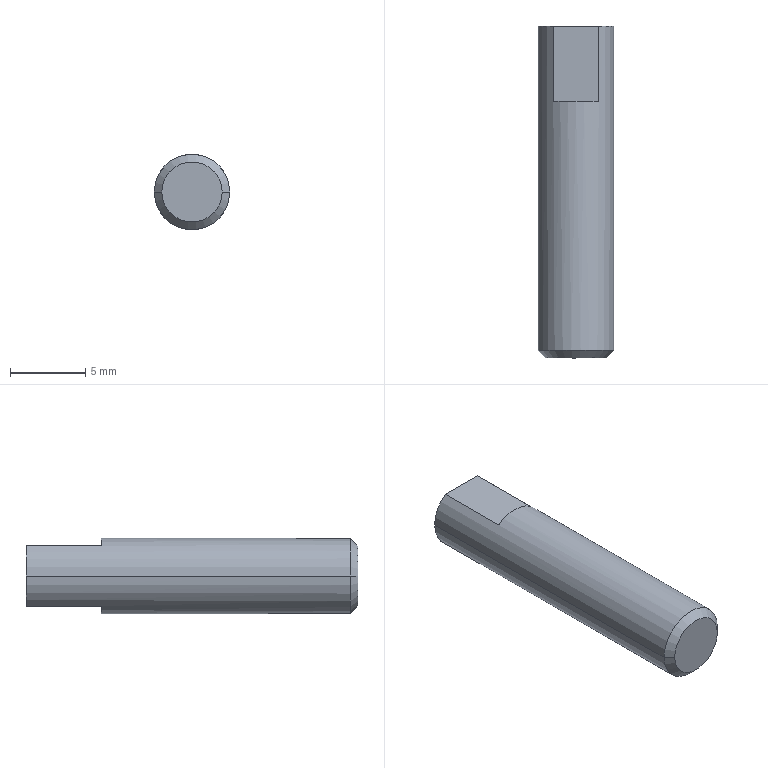Part | STEP file | BU-C08b-1 | 1 solid | 10 faces | box 5 x 22 x 5 mm | volume 419.918 mm3 | plane 6 | cone 2 | cylinder 2 | commonest cylinder face diameters 5 x2
STEP:
#1=CARTESIAN_POINT('',(0.,0.,0.));
#2=DIRECTION('',(0.,0.,1.));
#3=DIRECTION('',(1.,0.,0.));
#4=AXIS2_PLACEMENT_3D('',#1,#2,#3);
#5=CARTESIAN_POINT('',(2.,0.,0.));
#6=VERTEX_POINT('',#5);
#7=CARTESIAN_POINT('',(-2.,0.,0.));
#8=VERTEX_POINT('',#7);
#9=CARTESIAN_POINT('',(0.,0.,0.));
#10=DIRECTION('',(0.,-1.,0.));
#11=DIRECTION('',(1.,0.,0.));
#12=AXIS2_PLACEMENT_3D('',#9,#10,#11);
#13=CIRCLE('',#12,2.);
#14=CARTESIAN_POINT('',(0.,0.,0.));
#15=DIRECTION('',(0.,1.,0.));
#16=DIRECTION('',(-1.,0.,0.));
#17=AXIS2_PLACEMENT_3D('',#14,#15,#16);
#18=CONICAL_SURFACE('',#17,2.,0.7854);
#19=CARTESIAN_POINT('',(3.142,0.));
#20=DIRECTION('',(-1.,0.));
#21=VECTOR('',#20,1.);
#22=LINE('',#19,#21);
#23=(GEOMETRIC_REPRESENTATION_CONTEXT(2)PARAMETRIC_REPRESENTATION_CONTEXT()REPRESENTATION_CONTEXT('',''));
#24=DEFINITIONAL_REPRESENTATION('',(#22),#23);
#25=PCURVE('',#18,#24);
#26=CARTESIAN_POINT('',(0.,0.,0.));
#27=DIRECTION('',(0.,-1.,0.));
#28=DIRECTION('',(1.,0.,0.));
#29=AXIS2_PLACEMENT_3D('',#26,#27,#28);
#30=PLANE('',#29);
#31=CARTESIAN_POINT('',(0.,0.));
#32=DIRECTION('',(1.,0.));
#33=AXIS2_PLACEMENT_2D('',#31,#32);
#34=CIRCLE('',#33,2.);
#35=(GEOMETRIC_REPRESENTATION_CONTEXT(2)PARAMETRIC_REPRESENTATION_CONTEXT()REPRESENTATION_CONTEXT('',''));
#36=DEFINITIONAL_REPRESENTATION('',(#34),#35);
#37=PCURVE('',#30,#36);
#38=SURFACE_CURVE('',#13,(#25,#37),.PCURVE_S1.);
#39=EDGE_CURVE('',#6,#8,#38,.T.);
#40=ORIENTED_EDGE('',*,*,#39,.F.);
#41=CARTESIAN_POINT('',(2.5,0.5,0.));
#42=VERTEX_POINT('',#41);
#43=CARTESIAN_POINT('',(2.,0.,0.));
#44=DIRECTION('',(0.7071,0.7071,0.));
#45=VECTOR('',#44,1.);
#46=LINE('',#43,#45);
#47=CARTESIAN_POINT('',(3.142,0.));
#48=DIRECTION('',(0.,1.));
#49=VECTOR('',#48,1.);
#50=LINE('',#47,#49);
#51=(GEOMETRIC_REPRESENTATION_CONTEXT(2)PARAMETRIC_REPRESENTATION_CONTEXT()REPRESENTATION_CONTEXT('',''));
#52=DEFINITIONAL_REPRESENTATION('',(#50),#51);
#53=PCURVE('',#18,#52);
#54=CARTESIAN_POINT('',(0.,0.,0.));
#55=DIRECTION('',(0.,1.,0.));
#56=DIRECTION('',(-1.,0.,0.));
#57=AXIS2_PLACEMENT_3D('',#54,#55,#56);
#58=CONICAL_SURFACE('',#57,2.,0.7854);
#59=CARTESIAN_POINT('',(3.142,0.));
#60=DIRECTION('',(0.,1.));
#61=VECTOR('',#60,1.);
#62=LINE('',#59,#61);
#63=(GEOMETRIC_REPRESENTATION_CONTEXT(2)PARAMETRIC_REPRESENTATION_CONTEXT()REPRESENTATION_CONTEXT('',''));
#64=DEFINITIONAL_REPRESENTATION('',(#62),#63);
#65=PCURVE('',#58,#64);
#66=SURFACE_CURVE('',#46,(#53,#65),.PCURVE_S1.);
#67=EDGE_CURVE('',#6,#42,#66,.T.);
#68=ORIENTED_EDGE('',*,*,#67,.T.);
#69=CARTESIAN_POINT('',(-2.5,0.5,0.));
#70=VERTEX_POINT('',#69);
#71=CARTESIAN_POINT('',(0.,0.5,0.));
#72=DIRECTION('',(0.,1.,0.));
#73=DIRECTION('',(1.,0.,0.));
#74=AXIS2_PLACEMENT_3D('',#71,#72,#73);
#75=CIRCLE('',#74,2.5);
#76=CARTESIAN_POINT('',(-3.142,0.5));
#77=DIRECTION('',(1.,0.));
#78=VECTOR('',#77,1.);
#79=LINE('',#76,#78);
#80=(GEOMETRIC_REPRESENTATION_CONTEXT(2)PARAMETRIC_REPRESENTATION_CONTEXT()REPRESENTATION_CONTEXT('',''));
#81=DEFINITIONAL_REPRESENTATION('',(#79),#80);
#82=PCURVE('',#18,#81);
#83=CARTESIAN_POINT('',(0.,-1000.,0.));
#84=DIRECTION('',(0.,-1.,0.));
#85=DIRECTION('',(1.,0.,0.));
#86=AXIS2_PLACEMENT_3D('',#83,#84,#85);
#87=CYLINDRICAL_SURFACE('',#86,2.5);
#88=CARTESIAN_POINT('',(6.283,-1000.5));
#89=DIRECTION('',(-1.,0.));
#90=VECTOR('',#89,1.);
#91=LINE('',#88,#90);
#92=(GEOMETRIC_REPRESENTATION_CONTEXT(2)PARAMETRIC_REPRESENTATION_CONTEXT()REPRESENTATION_CONTEXT('',''));
#93=DEFINITIONAL_REPRESENTATION('',(#91),#92);
#94=PCURVE('',#87,#93);
#95=SURFACE_CURVE('',#75,(#82,#94),.PCURVE_S1.);
#96=EDGE_CURVE('',#70,#42,#95,.T.);
#97=ORIENTED_EDGE('',*,*,#96,.F.);
#98=CARTESIAN_POINT('',(-2.,0.,0.));
#99=DIRECTION('',(-0.7071,0.7071,0.));
#100=VECTOR('',#99,1.);
#101=LINE('',#98,#100);
#102=CARTESIAN_POINT('',(0.,0.));
#103=DIRECTION('',(0.,1.));
#104=VECTOR('',#103,1.);
#105=LINE('',#102,#104);
#106=(GEOMETRIC_REPRESENTATION_CONTEXT(2)PARAMETRIC_REPRESENTATION_CONTEXT()REPRESENTATION_CONTEXT('',''));
#107=DEFINITIONAL_REPRESENTATION('',(#105),#106);
#108=PCURVE('',#18,#107);
#109=CARTESIAN_POINT('',(6.283,0.));
#110=DIRECTION('',(0.,1.));
#111=VECTOR('',#110,1.);
#112=LINE('',#109,#111);
#113=(GEOMETRIC_REPRESENTATION_CONTEXT(2)PARAMETRIC_REPRESENTATION_CONTEXT()REPRESENTATION_CONTEXT('',''));
#114=DEFINITIONAL_REPRESENTATION('',(#112),#113);
#115=PCURVE('',#58,#114);
#116=SURFACE_CURVE('',#101,(#108,#115),.PCURVE_S1.);
#117=EDGE_CURVE('',#8,#70,#116,.T.);
#118=ORIENTED_EDGE('',*,*,#117,.F.);
#119=EDGE_LOOP('',(#40,#68,#97,#118));
#120=FACE_BOUND('',#119,.T.);
#121=ADVANCED_FACE('',(#120),#18,.T.);
#122=CARTESIAN_POINT('',(-1.5,22.,2.));
#123=VERTEX_POINT('',#122);
#124=CARTESIAN_POINT('',(-2.5,22.,0.));
#125=VERTEX_POINT('',#124);
#126=CARTESIAN_POINT('',(0.,22.,0.));
#127=DIRECTION('',(0.,-1.,0.));
#128=DIRECTION('',(1.,0.,0.));
#129=AXIS2_PLACEMENT_3D('',#126,#127,#128);
#130=CIRCLE('',#129,2.5);
#131=CARTESIAN_POINT('',(0.,-1022.));
#132=DIRECTION('',(1.,0.));
#133=VECTOR('',#132,1.);
#134=LINE('',#131,#133);
#135=(GEOMETRIC_REPRESENTATION_CONTEXT(2)PARAMETRIC_REPRESENTATION_CONTEXT()REPRESENTATION_CONTEXT('',''));
#136=DEFINITIONAL_REPRESENTATION('',(#134),#135);
#137=PCURVE('',#87,#136);
#138=CARTESIAN_POINT('',(0.,22.,0.));
#139=DIRECTION('',(0.,1.,0.));
#140=DIRECTION('',(-1.,0.,0.));
#141=AXIS2_PLACEMENT_3D('',#138,#139,#140);
#142=PLANE('',#141);
#143=CARTESIAN_POINT('',(-2.5,0.));
#144=CARTESIAN_POINT('',(-2.5,4.33));
#145=CARTESIAN_POINT('',(1.25,2.165));
#146=CARTESIAN_POINT('',(5.,0.));
#147=CARTESIAN_POINT('',(1.25,-2.165));
#148=CARTESIAN_POINT('',(-2.5,-4.33));
#149=CARTESIAN_POINT('',(-2.5,0.));
#150=(BOUNDED_CURVE()B_SPLINE_CURVE(2,(#143,#144,#145,#146,#147,#148,#149),.UNSPECIFIED.,.T.,.F.)B_SPLINE_CURVE_WITH_KNOTS((1,2,2,2,2,1),(-2.094,0.,2.094,4.189,6.283,8.378),.UNSPECIFIED.)CURVE()GEOMETRIC_REPRESENTATION_ITEM()RATIONAL_B_SPLINE_CURVE((1.,0.5,1.,0.5,1.,0.5,1.))REPRESENTATION_ITEM(''));
#151=(GEOMETRIC_REPRESENTATION_CONTEXT(2)PARAMETRIC_REPRESENTATION_CONTEXT()REPRESENTATION_CONTEXT('',''));
#152=DEFINITIONAL_REPRESENTATION('',(#150),#151);
#153=PCURVE('',#142,#152);
#154=SURFACE_CURVE('',#130,(#137,#153),.PCURVE_S1.);
#155=EDGE_CURVE('',#123,#125,#154,.T.);
#156=ORIENTED_EDGE('',*,*,#155,.T.);
#157=CARTESIAN_POINT('',(-2.5,-1000.,0.));
#158=DIRECTION('',(0.,-1.,0.));
#159=VECTOR('',#158,1.);
#160=LINE('',#157,#159);
#161=CARTESIAN_POINT('',(3.142,0.));
#162=DIRECTION('',(0.,1.));
#163=VECTOR('',#162,1.);
#164=LINE('',#161,#163);
#165=(GEOMETRIC_REPRESENTATION_CONTEXT(2)PARAMETRIC_REPRESENTATION_CONTEXT()REPRESENTATION_CONTEXT('',''));
#166=DEFINITIONAL_REPRESENTATION('',(#164),#165);
#167=PCURVE('',#87,#166);
#168=CARTESIAN_POINT('',(0.,-1000.,0.));
#169=DIRECTION('',(0.,-1.,0.));
#170=DIRECTION('',(1.,0.,0.));
#171=AXIS2_PLACEMENT_3D('',#168,#169,#170);
#172=CYLINDRICAL_SURFACE('',#171,2.5);
#173=CARTESIAN_POINT('',(3.142,0.));
#174=DIRECTION('',(0.,1.));
#175=VECTOR('',#174,1.);
#176=LINE('',#173,#175);
#177=(GEOMETRIC_REPRESENTATION_CONTEXT(2)PARAMETRIC_REPRESENTATION_CONTEXT()REPRESENTATION_CONTEXT('',''));
#178=DEFINITIONAL_REPRESENTATION('',(#176),#177);
#179=PCURVE('',#172,#178);
#180=SURFACE_CURVE('',#160,(#167,#179),.PCURVE_S1.);
#181=EDGE_CURVE('',#125,#70,#180,.T.);
#182=ORIENTED_EDGE('',*,*,#181,.T.);
#183=ORIENTED_EDGE('',*,*,#96,.T.);
#184=CARTESIAN_POINT('',(2.5,22.,0.));
#185=VERTEX_POINT('',#184);
#186=CARTESIAN_POINT('',(2.5,-1000.,0.));
#187=DIRECTION('',(0.,-1.,0.));
#188=VECTOR('',#187,1.);
#189=LINE('',#186,#188);
#190=CARTESIAN_POINT('',(0.,0.));
#191=DIRECTION('',(0.,1.));
#192=VECTOR('',#191,1.);
#193=LINE('',#190,#192);
#194=(GEOMETRIC_REPRESENTATION_CONTEXT(2)PARAMETRIC_REPRESENTATION_CONTEXT()REPRESENTATION_CONTEXT('',''));
#195=DEFINITIONAL_REPRESENTATION('',(#193),#194);
#196=PCURVE('',#87,#195);
#197=CARTESIAN_POINT('',(6.283,0.));
#198=DIRECTION('',(0.,1.));
#199=VECTOR('',#198,1.);
#200=LINE('',#197,#199);
#201=(GEOMETRIC_REPRESENTATION_CONTEXT(2)PARAMETRIC_REPRESENTATION_CONTEXT()REPRESENTATION_CONTEXT('',''));
#202=DEFINITIONAL_REPRESENTATION('',(#200),#201);
#203=PCURVE('',#172,#202);
#204=SURFACE_CURVE('',#189,(#196,#203),.PCURVE_S1.);
#205=EDGE_CURVE('',#185,#42,#204,.T.);
#206=ORIENTED_EDGE('',*,*,#205,.F.);
#207=CARTESIAN_POINT('',(1.5,22.,2.));
#208=VERTEX_POINT('',#207);
#209=CARTESIAN_POINT('',(0.,22.,0.));
#210=DIRECTION('',(0.,-1.,0.));
#211=DIRECTION('',(1.,0.,0.));
#212=AXIS2_PLACEMENT_3D('',#209,#210,#211);
#213=CIRCLE('',#212,2.5);
#214=CARTESIAN_POINT('',(0.,-1022.));
#215=DIRECTION('',(1.,0.));
#216=VECTOR('',#215,1.);
#217=LINE('',#214,#216);
#218=(GEOMETRIC_REPRESENTATION_CONTEXT(2)PARAMETRIC_REPRESENTATION_CONTEXT()REPRESENTATION_CONTEXT('',''));
#219=DEFINITIONAL_REPRESENTATION('',(#217),#218);
#220=PCURVE('',#87,#219);
#221=CARTESIAN_POINT('',(-2.5,0.));
#222=CARTESIAN_POINT('',(-2.5,4.33));
#223=CARTESIAN_POINT('',(1.25,2.165));
#224=CARTESIAN_POINT('',(5.,0.));
#225=CARTESIAN_POINT('',(1.25,-2.165));
#226=CARTESIAN_POINT('',(-2.5,-4.33));
#227=CARTESIAN_POINT('',(-2.5,0.));
#228=(BOUNDED_CURVE()B_SPLINE_CURVE(2,(#221,#222,#223,#224,#225,#226,#227),.UNSPECIFIED.,.T.,.F.)B_SPLINE_CURVE_WITH_KNOTS((1,2,2,2,2,1),(-2.094,0.,2.094,4.189,6.283,8.378),.UNSPECIFIED.)CURVE()GEOMETRIC_REPRESENTATION_ITEM()RATIONAL_B_SPLINE_CURVE((1.,0.5,1.,0.5,1.,0.5,1.))REPRESENTATION_ITEM(''));
#229=(GEOMETRIC_REPRESENTATION_CONTEXT(2)PARAMETRIC_REPRESENTATION_CONTEXT()REPRESENTATION_CONTEXT('',''));
#230=DEFINITIONAL_REPRESENTATION('',(#228),#229);
#231=PCURVE('',#142,#230);
#232=SURFACE_CURVE('',#213,(#220,#231),.PCURVE_S1.);
#233=EDGE_CURVE('',#185,#208,#232,.T.);
#234=ORIENTED_EDGE('',*,*,#233,.T.);
#235=CARTESIAN_POINT('',(1.5,17.,2.));
#236=VERTEX_POINT('',#235);
#237=CARTESIAN_POINT('',(1.5,17.,2.));
#238=DIRECTION('',(0.,1.,0.));
#239=VECTOR('',#238,1.);
#240=LINE('',#237,#239);
#241=CARTESIAN_POINT('',(0.9273,-1017.));
#242=DIRECTION('',(0.,-1.));
#243=VECTOR('',#242,1.);
#244=LINE('',#241,#243);
#245=(GEOMETRIC_REPRESENTATION_CONTEXT(2)PARAMETRIC_REPRESENTATION_CONTEXT()REPRESENTATION_CONTEXT('',''));
#246=DEFINITIONAL_REPRESENTATION('',(#244),#245);
#247=PCURVE('',#87,#246);
#248=CARTESIAN_POINT('',(-1.5,17.,2.));
#249=DIRECTION('',(0.,0.,-1.));
#250=DIRECTION('',(-1.,0.,0.));
#251=AXIS2_PLACEMENT_3D('',#248,#249,#250);
#252=PLANE('',#251);
#253=CARTESIAN_POINT('',(-3.,0.));
#254=DIRECTION('',(0.,1.));
#255=VECTOR('',#254,1.);
#256=LINE('',#253,#255);
#257=(GEOMETRIC_REPRESENTATION_CONTEXT(2)PARAMETRIC_REPRESENTATION_CONTEXT()REPRESENTATION_CONTEXT('',''));
#258=DEFINITIONAL_REPRESENTATION('',(#256),#257);
#259=PCURVE('',#252,#258);
#260=SURFACE_CURVE('',#240,(#247,#259),.PCURVE_S1.);
#261=EDGE_CURVE('',#236,#208,#260,.T.);
#262=ORIENTED_EDGE('',*,*,#261,.F.);
#263=CARTESIAN_POINT('',(-1.5,17.,2.));
#264=VERTEX_POINT('',#263);
#265=CARTESIAN_POINT('',(0.,17.,0.));
#266=DIRECTION('',(0.,1.,0.));
#267=DIRECTION('',(-1.,0.,0.));
#268=AXIS2_PLACEMENT_3D('',#265,#266,#267);
#269=CIRCLE('',#268,2.5);
#270=CARTESIAN_POINT('',(3.142,-1017.));
#271=DIRECTION('',(-1.,0.));
#272=VECTOR('',#271,1.);
#273=LINE('',#270,#272);
#274=(GEOMETRIC_REPRESENTATION_CONTEXT(2)PARAMETRIC_REPRESENTATION_CONTEXT()REPRESENTATION_CONTEXT('',''));
#275=DEFINITIONAL_REPRESENTATION('',(#273),#274);
#276=PCURVE('',#87,#275);
#277=CARTESIAN_POINT('',(0.,17.,0.));
#278=DIRECTION('',(0.,1.,0.));
#279=DIRECTION('',(-1.,0.,0.));
#280=AXIS2_PLACEMENT_3D('',#277,#278,#279);
#281=PLANE('',#280);
#282=CARTESIAN_POINT('',(0.,0.));
#283=DIRECTION('',(1.,0.));
#284=AXIS2_PLACEMENT_2D('',#282,#283);
#285=CIRCLE('',#284,2.5);
#286=(GEOMETRIC_REPRESENTATION_CONTEXT(2)PARAMETRIC_REPRESENTATION_CONTEXT()REPRESENTATION_CONTEXT('',''));
#287=DEFINITIONAL_REPRESENTATION('',(#285),#286);
#288=PCURVE('',#281,#287);
#289=SURFACE_CURVE('',#269,(#276,#288),.PCURVE_S1.);
#290=EDGE_CURVE('',#264,#236,#289,.T.);
#291=ORIENTED_EDGE('',*,*,#290,.F.);
#292=CARTESIAN_POINT('',(-1.5,17.,2.));
#293=DIRECTION('',(0.,1.,0.));
#294=VECTOR('',#293,1.);
#295=LINE('',#292,#294);
#296=CARTESIAN_POINT('',(2.214,-1017.));
#297=DIRECTION('',(0.,-1.));
#298=VECTOR('',#297,1.);
#299=LINE('',#296,#298);
#300=(GEOMETRIC_REPRESENTATION_CONTEXT(2)PARAMETRIC_REPRESENTATION_CONTEXT()REPRESENTATION_CONTEXT('',''));
#301=DEFINITIONAL_REPRESENTATION('',(#299),#300);
#302=PCURVE('',#87,#301);
#303=CARTESIAN_POINT('',(0.,0.));
#304=DIRECTION('',(0.,1.));
#305=VECTOR('',#304,1.);
#306=LINE('',#303,#305);
#307=(GEOMETRIC_REPRESENTATION_CONTEXT(2)PARAMETRIC_REPRESENTATION_CONTEXT()REPRESENTATION_CONTEXT('',''));
#308=DEFINITIONAL_REPRESENTATION('',(#306),#307);
#309=PCURVE('',#252,#308);
#310=SURFACE_CURVE('',#295,(#302,#309),.PCURVE_S1.);
#311=EDGE_CURVE('',#264,#123,#310,.T.);
#312=ORIENTED_EDGE('',*,*,#311,.T.);
#313=EDGE_LOOP('',(#156,#182,#183,#206,#234,#262,#291,#312));
#314=FACE_BOUND('',#313,.T.);
#315=ADVANCED_FACE('',(#314),#87,.T.);
#316=CARTESIAN_POINT('',(-1.5,22.,2.));
#317=DIRECTION('',(-1.,0.,0.));
#318=VECTOR('',#317,1.);
#319=LINE('',#316,#318);
#320=CARTESIAN_POINT('',(1.5,2.));
#321=DIRECTION('',(1.,0.));
#322=VECTOR('',#321,1.);
#323=LINE('',#320,#322);
#324=(GEOMETRIC_REPRESENTATION_CONTEXT(2)PARAMETRIC_REPRESENTATION_CONTEXT()REPRESENTATION_CONTEXT('',''));
#325=DEFINITIONAL_REPRESENTATION('',(#323),#324);
#326=PCURVE('',#142,#325);
#327=CARTESIAN_POINT('',(0.,5.));
#328=DIRECTION('',(1.,0.));
#329=VECTOR('',#328,1.);
#330=LINE('',#327,#329);
#331=(GEOMETRIC_REPRESENTATION_CONTEXT(2)PARAMETRIC_REPRESENTATION_CONTEXT()REPRESENTATION_CONTEXT('',''));
#332=DEFINITIONAL_REPRESENTATION('',(#330),#331);
#333=PCURVE('',#252,#332);
#334=SURFACE_CURVE('',#319,(#326,#333),.PCURVE_S1.);
#335=EDGE_CURVE('',#208,#123,#334,.T.);
#336=ORIENTED_EDGE('',*,*,#335,.F.);
#337=ORIENTED_EDGE('',*,*,#233,.F.);
#338=CARTESIAN_POINT('',(1.5,22.,-2.));
#339=VERTEX_POINT('',#338);
#340=CARTESIAN_POINT('',(0.,22.,0.));
#341=DIRECTION('',(0.,-1.,0.));
#342=DIRECTION('',(1.,0.,0.));
#343=AXIS2_PLACEMENT_3D('',#340,#341,#342);
#344=CIRCLE('',#343,2.5);
#345=CARTESIAN_POINT('',(-2.5,0.));
#346=CARTESIAN_POINT('',(-2.5,4.33));
#347=CARTESIAN_POINT('',(1.25,2.165));
#348=CARTESIAN_POINT('',(5.,0.));
#349=CARTESIAN_POINT('',(1.25,-2.165));
#350=CARTESIAN_POINT('',(-2.5,-4.33));
#351=CARTESIAN_POINT('',(-2.5,0.));
#352=(BOUNDED_CURVE()B_SPLINE_CURVE(2,(#345,#346,#347,#348,#349,#350,#351),.UNSPECIFIED.,.T.,.F.)B_SPLINE_CURVE_WITH_KNOTS((1,2,2,2,2,1),(-2.094,0.,2.094,4.189,6.283,8.378),.UNSPECIFIED.)CURVE()GEOMETRIC_REPRESENTATION_ITEM()RATIONAL_B_SPLINE_CURVE((1.,0.5,1.,0.5,1.,0.5,1.))REPRESENTATION_ITEM(''));
#353=(GEOMETRIC_REPRESENTATION_CONTEXT(2)PARAMETRIC_REPRESENTATION_CONTEXT()REPRESENTATION_CONTEXT('',''));
#354=DEFINITIONAL_REPRESENTATION('',(#352),#353);
#355=PCURVE('',#142,#354);
#356=CARTESIAN_POINT('',(0.,-1022.));
#357=DIRECTION('',(1.,0.));
#358=VECTOR('',#357,1.);
#359=LINE('',#356,#358);
#360=(GEOMETRIC_REPRESENTATION_CONTEXT(2)PARAMETRIC_REPRESENTATION_CONTEXT()REPRESENTATION_CONTEXT('',''));
#361=DEFINITIONAL_REPRESENTATION('',(#359),#360);
#362=PCURVE('',#172,#361);
#363=SURFACE_CURVE('',#344,(#355,#362),.PCURVE_S1.);
#364=EDGE_CURVE('',#339,#185,#363,.T.);
#365=ORIENTED_EDGE('',*,*,#364,.F.);
#366=CARTESIAN_POINT('',(-1.5,22.,-2.));
#367=VERTEX_POINT('',#366);
#368=CARTESIAN_POINT('',(-1.5,22.,-2.));
#369=DIRECTION('',(1.,0.,0.));
#370=VECTOR('',#369,1.);
#371=LINE('',#368,#370);
#372=CARTESIAN_POINT('',(1.5,-2.));
#373=DIRECTION('',(-1.,0.));
#374=VECTOR('',#373,1.);
#375=LINE('',#372,#374);
#376=(GEOMETRIC_REPRESENTATION_CONTEXT(2)PARAMETRIC_REPRESENTATION_CONTEXT()REPRESENTATION_CONTEXT('',''));
#377=DEFINITIONAL_REPRESENTATION('',(#375),#376);
#378=PCURVE('',#142,#377);
#379=CARTESIAN_POINT('',(-1.5,17.,-2.));
#380=DIRECTION('',(0.,0.,1.));
#381=DIRECTION('',(1.,0.,0.));
#382=AXIS2_PLACEMENT_3D('',#379,#380,#381);
#383=PLANE('',#382);
#384=CARTESIAN_POINT('',(0.,5.));
#385=DIRECTION('',(1.,0.));
#386=VECTOR('',#385,1.);
#387=LINE('',#384,#386);
#388=(GEOMETRIC_REPRESENTATION_CONTEXT(2)PARAMETRIC_REPRESENTATION_CONTEXT()REPRESENTATION_CONTEXT('',''));
#389=DEFINITIONAL_REPRESENTATION('',(#387),#388);
#390=PCURVE('',#383,#389);
#391=SURFACE_CURVE('',#371,(#378,#390),.PCURVE_S1.);
#392=EDGE_CURVE('',#367,#339,#391,.T.);
#393=ORIENTED_EDGE('',*,*,#392,.F.);
#394=CARTESIAN_POINT('',(0.,22.,0.));
#395=DIRECTION('',(0.,-1.,0.));
#396=DIRECTION('',(1.,0.,0.));
#397=AXIS2_PLACEMENT_3D('',#394,#395,#396);
#398=CIRCLE('',#397,2.5);
#399=CARTESIAN_POINT('',(-2.5,0.));
#400=CARTESIAN_POINT('',(-2.5,4.33));
#401=CARTESIAN_POINT('',(1.25,2.165));
#402=CARTESIAN_POINT('',(5.,0.));
#403=CARTESIAN_POINT('',(1.25,-2.165));
#404=CARTESIAN_POINT('',(-2.5,-4.33));
#405=CARTESIAN_POINT('',(-2.5,0.));
#406=(BOUNDED_CURVE()B_SPLINE_CURVE(2,(#399,#400,#401,#402,#403,#404,#405),.UNSPECIFIED.,.T.,.F.)B_SPLINE_CURVE_WITH_KNOTS((1,2,2,2,2,1),(-2.094,0.,2.094,4.189,6.283,8.378),.UNSPECIFIED.)CURVE()GEOMETRIC_REPRESENTATION_ITEM()RATIONAL_B_SPLINE_CURVE((1.,0.5,1.,0.5,1.,0.5,1.))REPRESENTATION_ITEM(''));
#407=(GEOMETRIC_REPRESENTATION_CONTEXT(2)PARAMETRIC_REPRESENTATION_CONTEXT()REPRESENTATION_CONTEXT('',''));
#408=DEFINITIONAL_REPRESENTATION('',(#406),#407);
#409=PCURVE('',#142,#408);
#410=CARTESIAN_POINT('',(0.,-1022.));
#411=DIRECTION('',(1.,0.));
#412=VECTOR('',#411,1.);
#413=LINE('',#410,#412);
#414=(GEOMETRIC_REPRESENTATION_CONTEXT(2)PARAMETRIC_REPRESENTATION_CONTEXT()REPRESENTATION_CONTEXT('',''));
#415=DEFINITIONAL_REPRESENTATION('',(#413),#414);
#416=PCURVE('',#172,#415);
#417=SURFACE_CURVE('',#398,(#409,#416),.PCURVE_S1.);
#418=EDGE_CURVE('',#125,#367,#417,.T.);
#419=ORIENTED_EDGE('',*,*,#418,.F.);
#420=ORIENTED_EDGE('',*,*,#155,.F.);
#421=EDGE_LOOP('',(#336,#337,#365,#393,#419,#420));
#422=FACE_BOUND('',#421,.T.);
#423=ADVANCED_FACE('',(#422),#142,.T.);
#424=ORIENTED_EDGE('',*,*,#181,.F.);
#425=ORIENTED_EDGE('',*,*,#418,.T.);
#426=CARTESIAN_POINT('',(-1.5,17.,-2.));
#427=VERTEX_POINT('',#426);
#428=CARTESIAN_POINT('',(-1.5,17.,-2.));
#429=DIRECTION('',(0.,1.,0.));
#430=VECTOR('',#429,1.);
#431=LINE('',#428,#430);
#432=CARTESIAN_POINT('',(4.069,-1017.));
#433=DIRECTION('',(0.,-1.));
#434=VECTOR('',#433,1.);
#435=LINE('',#432,#434);
#436=(GEOMETRIC_REPRESENTATION_CONTEXT(2)PARAMETRIC_REPRESENTATION_CONTEXT()REPRESENTATION_CONTEXT('',''));
#437=DEFINITIONAL_REPRESENTATION('',(#435),#436);
#438=PCURVE('',#172,#437);
#439=CARTESIAN_POINT('',(0.,0.));
#440=DIRECTION('',(0.,1.));
#441=VECTOR('',#440,1.);
#442=LINE('',#439,#441);
#443=(GEOMETRIC_REPRESENTATION_CONTEXT(2)PARAMETRIC_REPRESENTATION_CONTEXT()REPRESENTATION_CONTEXT('',''));
#444=DEFINITIONAL_REPRESENTATION('',(#442),#443);
#445=PCURVE('',#383,#444);
#446=SURFACE_CURVE('',#431,(#438,#445),.PCURVE_S1.);
#447=EDGE_CURVE('',#427,#367,#446,.T.);
#448=ORIENTED_EDGE('',*,*,#447,.F.);
#449=CARTESIAN_POINT('',(1.5,17.,-2.));
#450=VERTEX_POINT('',#449);
#451=CARTESIAN_POINT('',(0.,17.,0.));
#452=DIRECTION('',(0.,1.,0.));
#453=DIRECTION('',(-1.,0.,0.));
#454=AXIS2_PLACEMENT_3D('',#451,#452,#453);
#455=CIRCLE('',#454,2.5);
#456=CARTESIAN_POINT('',(9.425,-1017.));
#457=DIRECTION('',(-1.,0.));
#458=VECTOR('',#457,1.);
#459=LINE('',#456,#458);
#460=(GEOMETRIC_REPRESENTATION_CONTEXT(2)PARAMETRIC_REPRESENTATION_CONTEXT()REPRESENTATION_CONTEXT('',''));
#461=DEFINITIONAL_REPRESENTATION('',(#459),#460);
#462=PCURVE('',#172,#461);
#463=CARTESIAN_POINT('',(0.,17.,0.));
#464=DIRECTION('',(0.,1.,0.));
#465=DIRECTION('',(-1.,0.,0.));
#466=AXIS2_PLACEMENT_3D('',#463,#464,#465);
#467=PLANE('',#466);
#468=CARTESIAN_POINT('',(0.,0.));
#469=DIRECTION('',(1.,0.));
#470=AXIS2_PLACEMENT_2D('',#468,#469);
#471=CIRCLE('',#470,2.5);
#472=(GEOMETRIC_REPRESENTATION_CONTEXT(2)PARAMETRIC_REPRESENTATION_CONTEXT()REPRESENTATION_CONTEXT('',''));
#473=DEFINITIONAL_REPRESENTATION('',(#471),#472);
#474=PCURVE('',#467,#473);
#475=SURFACE_CURVE('',#455,(#462,#474),.PCURVE_S1.);
#476=EDGE_CURVE('',#450,#427,#475,.T.);
#477=ORIENTED_EDGE('',*,*,#476,.F.);
#478=CARTESIAN_POINT('',(1.5,17.,-2.));
#479=DIRECTION('',(0.,1.,0.));
#480=VECTOR('',#479,1.);
#481=LINE('',#478,#480);
#482=CARTESIAN_POINT('',(5.356,-1017.));
#483=DIRECTION('',(0.,-1.));
#484=VECTOR('',#483,1.);
#485=LINE('',#482,#484);
#486=(GEOMETRIC_REPRESENTATION_CONTEXT(2)PARAMETRIC_REPRESENTATION_CONTEXT()REPRESENTATION_CONTEXT('',''));
#487=DEFINITIONAL_REPRESENTATION('',(#485),#486);
#488=PCURVE('',#172,#487);
#489=CARTESIAN_POINT('',(3.,0.));
#490=DIRECTION('',(0.,1.));
#491=VECTOR('',#490,1.);
#492=LINE('',#489,#491);
#493=(GEOMETRIC_REPRESENTATION_CONTEXT(2)PARAMETRIC_REPRESENTATION_CONTEXT()REPRESENTATION_CONTEXT('',''));
#494=DEFINITIONAL_REPRESENTATION('',(#492),#493);
#495=PCURVE('',#383,#494);
#496=SURFACE_CURVE('',#481,(#488,#495),.PCURVE_S1.);
#497=EDGE_CURVE('',#450,#339,#496,.T.);
#498=ORIENTED_EDGE('',*,*,#497,.T.);
#499=ORIENTED_EDGE('',*,*,#364,.T.);
#500=ORIENTED_EDGE('',*,*,#205,.T.);
#501=CARTESIAN_POINT('',(0.,0.5,0.));
#502=DIRECTION('',(0.,1.,0.));
#503=DIRECTION('',(1.,0.,0.));
#504=AXIS2_PLACEMENT_3D('',#501,#502,#503);
#505=CIRCLE('',#504,2.5);
#506=CARTESIAN_POINT('',(6.283,-1000.5));
#507=DIRECTION('',(-1.,0.));
#508=VECTOR('',#507,1.);
#509=LINE('',#506,#508);
#510=(GEOMETRIC_REPRESENTATION_CONTEXT(2)PARAMETRIC_REPRESENTATION_CONTEXT()REPRESENTATION_CONTEXT('',''));
#511=DEFINITIONAL_REPRESENTATION('',(#509),#510);
#512=PCURVE('',#172,#511);
#513=CARTESIAN_POINT('',(3.142,0.5));
#514=DIRECTION('',(1.,0.));
#515=VECTOR('',#514,1.);
#516=LINE('',#513,#515);
#517=(GEOMETRIC_REPRESENTATION_CONTEXT(2)PARAMETRIC_REPRESENTATION_CONTEXT()REPRESENTATION_CONTEXT('',''));
#518=DEFINITIONAL_REPRESENTATION('',(#516),#517);
#519=PCURVE('',#58,#518);
#520=SURFACE_CURVE('',#505,(#512,#519),.PCURVE_S1.);
#521=EDGE_CURVE('',#42,#70,#520,.T.);
#522=ORIENTED_EDGE('',*,*,#521,.T.);
#523=EDGE_LOOP('',(#424,#425,#448,#477,#498,#499,#500,#522));
#524=FACE_BOUND('',#523,.T.);
#525=ADVANCED_FACE('',(#524),#172,.T.);
#526=CARTESIAN_POINT('',(0.,0.,0.));
#527=DIRECTION('',(0.,-1.,0.));
#528=DIRECTION('',(1.,0.,0.));
#529=AXIS2_PLACEMENT_3D('',#526,#527,#528);
#530=CIRCLE('',#529,2.);
#531=CARTESIAN_POINT('',(0.,0.));
#532=DIRECTION('',(1.,0.));
#533=AXIS2_PLACEMENT_2D('',#531,#532);
#534=CIRCLE('',#533,2.);
#535=(GEOMETRIC_REPRESENTATION_CONTEXT(2)PARAMETRIC_REPRESENTATION_CONTEXT()REPRESENTATION_CONTEXT('',''));
#536=DEFINITIONAL_REPRESENTATION('',(#534),#535);
#537=PCURVE('',#30,#536);
#538=CARTESIAN_POINT('',(9.425,0.));
#539=DIRECTION('',(-1.,0.));
#540=VECTOR('',#539,1.);
#541=LINE('',#538,#540);
#542=(GEOMETRIC_REPRESENTATION_CONTEXT(2)PARAMETRIC_REPRESENTATION_CONTEXT()REPRESENTATION_CONTEXT('',''));
#543=DEFINITIONAL_REPRESENTATION('',(#541),#542);
#544=PCURVE('',#58,#543);
#545=SURFACE_CURVE('',#530,(#537,#544),.PCURVE_S1.);
#546=EDGE_CURVE('',#8,#6,#545,.T.);
#547=ORIENTED_EDGE('',*,*,#546,.T.);
#548=ORIENTED_EDGE('',*,*,#39,.T.);
#549=EDGE_LOOP('',(#547,#548));
#550=FACE_BOUND('',#549,.T.);
#551=ADVANCED_FACE('',(#550),#30,.T.);
#552=ORIENTED_EDGE('',*,*,#392,.T.);
#553=ORIENTED_EDGE('',*,*,#497,.F.);
#554=CARTESIAN_POINT('',(-1.5,17.,-2.));
#555=DIRECTION('',(1.,0.,0.));
#556=VECTOR('',#555,1.);
#557=LINE('',#554,#556);
#558=CARTESIAN_POINT('',(0.,0.));
#559=DIRECTION('',(1.,0.));
#560=VECTOR('',#559,1.);
#561=LINE('',#558,#560);
#562=(GEOMETRIC_REPRESENTATION_CONTEXT(2)PARAMETRIC_REPRESENTATION_CONTEXT()REPRESENTATION_CONTEXT('',''));
#563=DEFINITIONAL_REPRESENTATION('',(#561),#562);
#564=PCURVE('',#383,#563);
#565=CARTESIAN_POINT('',(1.5,-2.));
#566=DIRECTION('',(-1.,0.));
#567=VECTOR('',#566,1.);
#568=LINE('',#565,#567);
#569=(GEOMETRIC_REPRESENTATION_CONTEXT(2)PARAMETRIC_REPRESENTATION_CONTEXT()REPRESENTATION_CONTEXT('',''));
#570=DEFINITIONAL_REPRESENTATION('',(#568),#569);
#571=PCURVE('',#467,#570);
#572=SURFACE_CURVE('',#557,(#564,#571),.PCURVE_S1.);
#573=EDGE_CURVE('',#427,#450,#572,.T.);
#574=ORIENTED_EDGE('',*,*,#573,.F.);
#575=ORIENTED_EDGE('',*,*,#447,.T.);
#576=EDGE_LOOP('',(#552,#553,#574,#575));
#577=FACE_BOUND('',#576,.T.);
#578=ADVANCED_FACE('',(#577),#383,.F.);
#579=ORIENTED_EDGE('',*,*,#476,.T.);
#580=ORIENTED_EDGE('',*,*,#573,.T.);
#581=EDGE_LOOP('',(#579,#580));
#582=FACE_BOUND('',#581,.T.);
#583=ADVANCED_FACE('',(#582),#467,.T.);
#584=ORIENTED_EDGE('',*,*,#335,.T.);
#585=ORIENTED_EDGE('',*,*,#311,.F.);
#586=CARTESIAN_POINT('',(-1.5,17.,2.));
#587=DIRECTION('',(-1.,0.,0.));
#588=VECTOR('',#587,1.);
#589=LINE('',#586,#588);
#590=CARTESIAN_POINT('',(0.,0.));
#591=DIRECTION('',(1.,0.));
#592=VECTOR('',#591,1.);
#593=LINE('',#590,#592);
#594=(GEOMETRIC_REPRESENTATION_CONTEXT(2)PARAMETRIC_REPRESENTATION_CONTEXT()REPRESENTATION_CONTEXT('',''));
#595=DEFINITIONAL_REPRESENTATION('',(#593),#594);
#596=PCURVE('',#252,#595);
#597=CARTESIAN_POINT('',(1.5,2.));
#598=DIRECTION('',(1.,0.));
#599=VECTOR('',#598,1.);
#600=LINE('',#597,#599);
#601=(GEOMETRIC_REPRESENTATION_CONTEXT(2)PARAMETRIC_REPRESENTATION_CONTEXT()REPRESENTATION_CONTEXT('',''));
#602=DEFINITIONAL_REPRESENTATION('',(#600),#601);
#603=PCURVE('',#281,#602);
#604=SURFACE_CURVE('',#589,(#596,#603),.PCURVE_S1.);
#605=EDGE_CURVE('',#236,#264,#604,.T.);
#606=ORIENTED_EDGE('',*,*,#605,.F.);
#607=ORIENTED_EDGE('',*,*,#261,.T.);
#608=EDGE_LOOP('',(#584,#585,#606,#607));
#609=FACE_BOUND('',#608,.T.);
#610=ADVANCED_FACE('',(#609),#252,.F.);
#611=ORIENTED_EDGE('',*,*,#290,.T.);
#612=ORIENTED_EDGE('',*,*,#605,.T.);
#613=EDGE_LOOP('',(#611,#612));
#614=FACE_BOUND('',#613,.T.);
#615=ADVANCED_FACE('',(#614),#281,.T.);
#616=ORIENTED_EDGE('',*,*,#67,.F.);
#617=ORIENTED_EDGE('',*,*,#546,.F.);
#618=ORIENTED_EDGE('',*,*,#117,.T.);
#619=ORIENTED_EDGE('',*,*,#521,.F.);
#620=EDGE_LOOP('',(#616,#617,#618,#619));
#621=FACE_BOUND('',#620,.T.);
#622=ADVANCED_FACE('',(#621),#58,.T.);
#623=CLOSED_SHELL('',(#121,#315,#423,#525,#551,#578,#583,#610,#615,#622));
#624=MANIFOLD_SOLID_BREP('',#623);
#625=(LENGTH_UNIT()NAMED_UNIT(*)SI_UNIT(.MILLI.,.METRE.));
#626=UNCERTAINTY_MEASURE_WITH_UNIT(LENGTH_MEASURE(0.0000001),#625,'','');
#627=(NAMED_UNIT(*)PLANE_ANGLE_UNIT()SI_UNIT($,.RADIAN.));
#628=(NAMED_UNIT(*)SI_UNIT($,.STERADIAN.)SOLID_ANGLE_UNIT());
#629=(GEOMETRIC_REPRESENTATION_CONTEXT(3)GLOBAL_UNCERTAINTY_ASSIGNED_CONTEXT((#626))GLOBAL_UNIT_ASSIGNED_CONTEXT((#625,#627,#628))REPRESENTATION_CONTEXT('',''));
#630=ADVANCED_BREP_SHAPE_REPRESENTATION('',(#4,#624),#629);